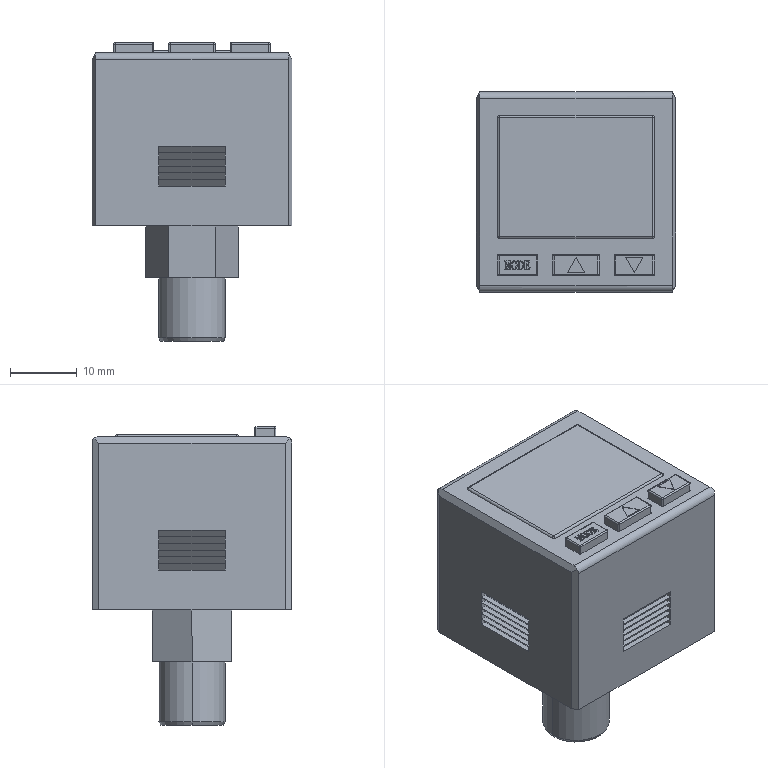Part | STEP file | 1 solid | 299 faces | box 30 x 30 x 44.8 mm | volume 24470 mm3 | plane 207 | cylinder 38 | spline 30 | sphere 16 | cone 8 | commonest cylinder face diameters 0.4 x24 0.6 x4 2.5 x4 2 x2 4 x2 10 x2